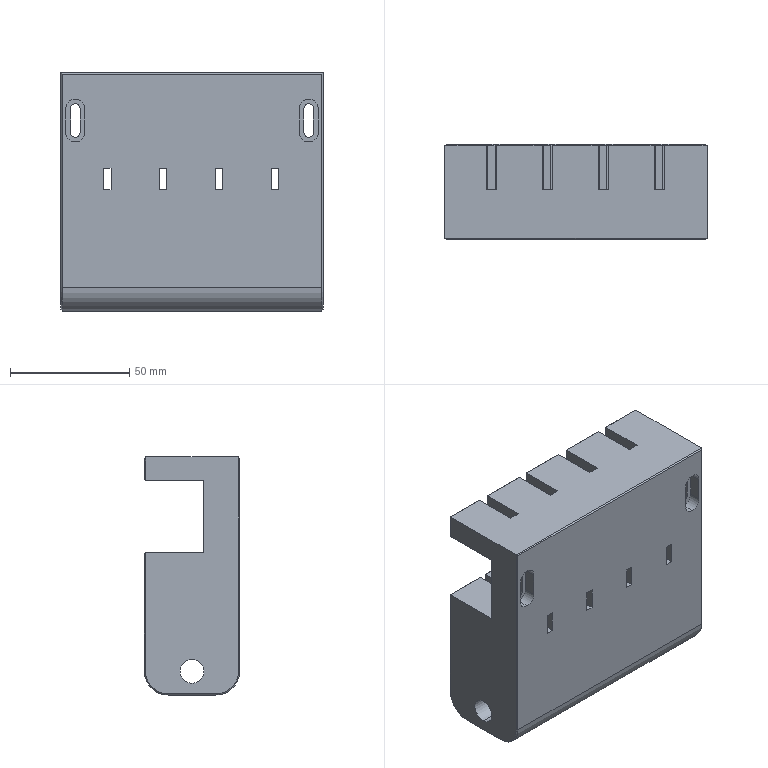Part | SolidWorks | features ICE 7, Chamfer 3, Extrusion 1, Fillet 1, HoleWzd 1 | 1 solid | 128 faces | box 110 x 40 x 100 mm | volume 333751 mm3 | plane 102 | cylinder 22 | cone 4 | commonest cylinder face diameters 4 x8 8 x6 6 x4 10 x2 20 x2